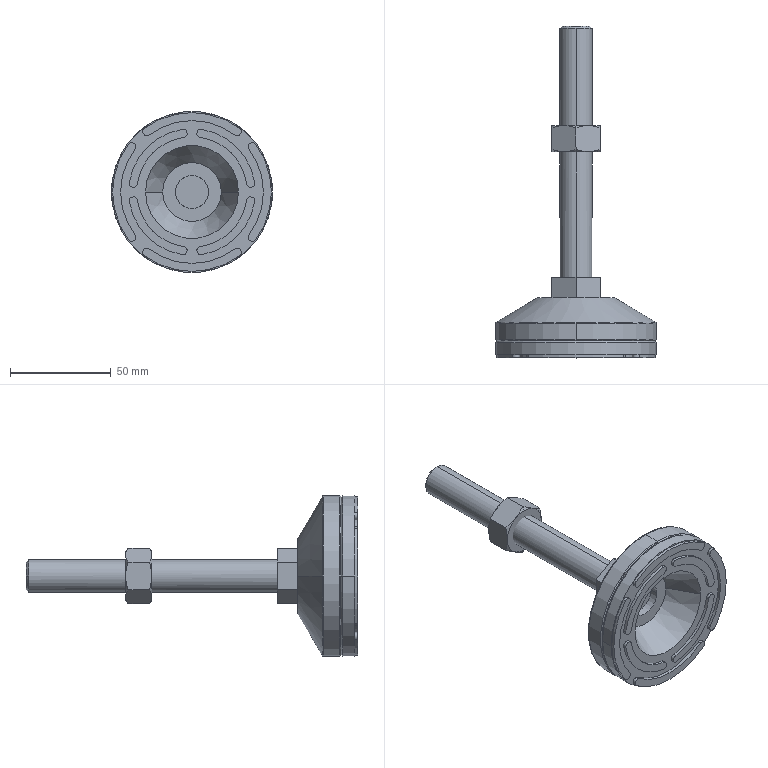Part | STEP file | E-WAC53-D80-M16-L125 | 3 solids | 112 faces | box 80 x 165 x 80 mm | volume 107171 mm3 | cylinder 56 | plane 32 | cone 22 | spline 2 | commonest cylinder face diameters 4 x24 71 x5 79 x5 16.5 x4 55 x4 63 x4